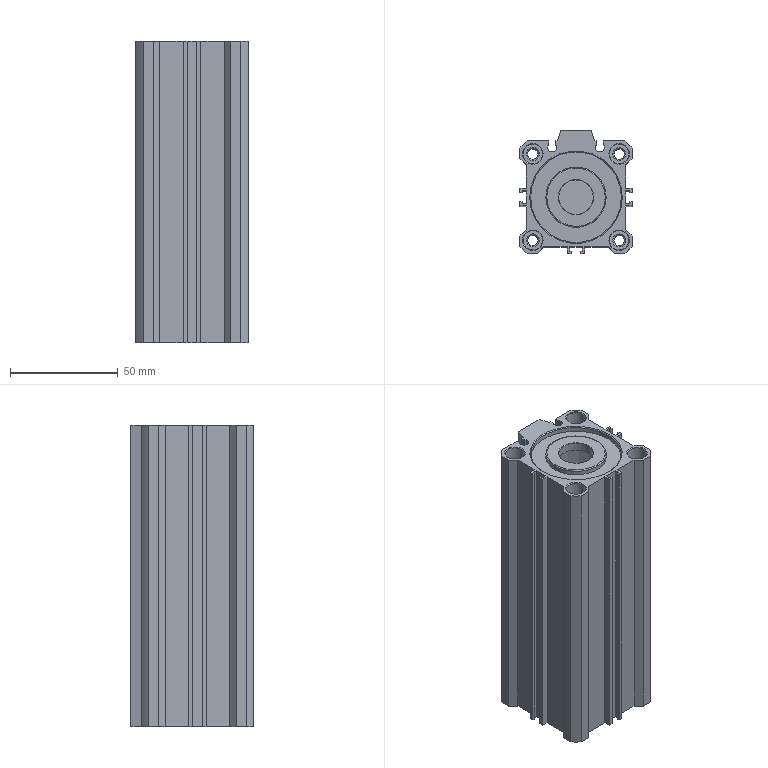Part | STEP file | HI_JSNR40X100_body_default | 1 solid | 186 faces | box 52 x 57 x 139.5 mm | volume 157789 mm3 | plane 88 | cylinder 48 | cone 46 | spline 4 | commonest cylinder face diameters 9 x16 4.917 x8 3 x4 28 x4 42 x4 69 x4